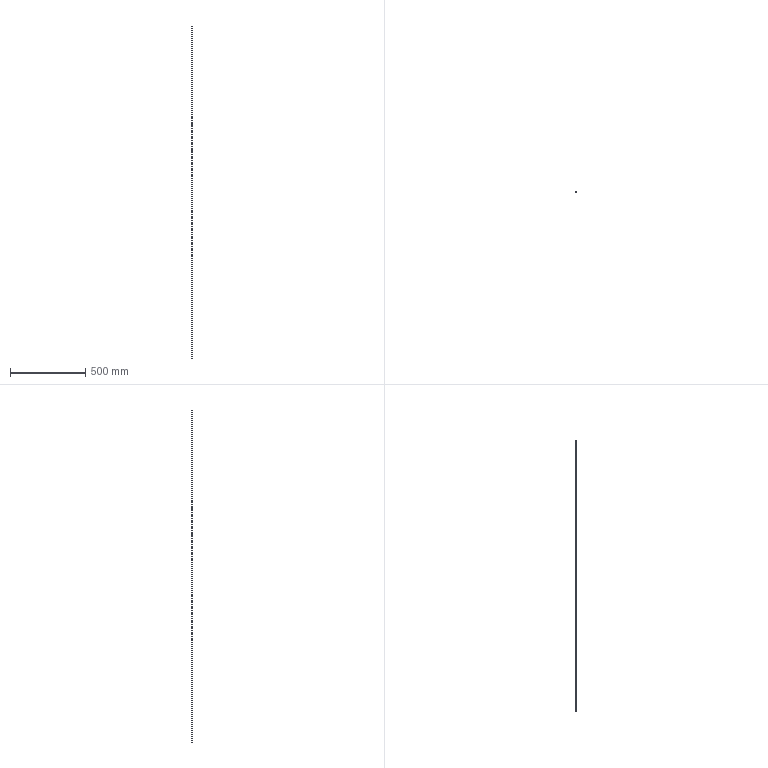Part | STEP file | P2 | 1 solid | 3 faces | box 4 x 4 x 2200 mm | volume 27646 mm3 | plane 2 | cylinder 1 | commonest cylinder face diameters 4 x1
STEP:
#1=CARTESIAN_POINT('',(0.,0.,0.));
#2=DIRECTION('',(0.,0.,1.));
#3=DIRECTION('',(1.,0.,0.));
#4=AXIS2_PLACEMENT_3D('',#1,#2,#3);
#5=CARTESIAN_POINT('',(2.,0.,2200.));
#6=VERTEX_POINT('',#5);
#7=CARTESIAN_POINT('',(0.,0.,2200.));
#8=DIRECTION('',(0.,0.,-1.));
#9=DIRECTION('',(-1.,0.,0.));
#10=AXIS2_PLACEMENT_3D('',#7,#8,#9);
#11=CIRCLE('',#10,2.);
#12=CARTESIAN_POINT('',(0.,0.,0.));
#13=DIRECTION('',(0.,0.,1.));
#14=DIRECTION('',(-1.,0.,0.));
#15=AXIS2_PLACEMENT_3D('',#12,#13,#14);
#16=CYLINDRICAL_SURFACE('',#15,2.);
#17=CARTESIAN_POINT('',(12.566,2200.));
#18=DIRECTION('',(-1.,0.));
#19=VECTOR('',#18,1.);
#20=LINE('',#17,#19);
#21=(GEOMETRIC_REPRESENTATION_CONTEXT(2)PARAMETRIC_REPRESENTATION_CONTEXT()REPRESENTATION_CONTEXT('',''));
#22=DEFINITIONAL_REPRESENTATION('',(#20),#21);
#23=PCURVE('',#16,#22);
#24=CARTESIAN_POINT('',(0.,0.,2200.));
#25=DIRECTION('',(0.,0.,1.));
#26=DIRECTION('',(1.,0.,0.));
#27=AXIS2_PLACEMENT_3D('',#24,#25,#26);
#28=PLANE('',#27);
#29=CARTESIAN_POINT('',(-2.,0.));
#30=CARTESIAN_POINT('',(-2.,3.464));
#31=CARTESIAN_POINT('',(1.,1.732));
#32=CARTESIAN_POINT('',(4.,0.));
#33=CARTESIAN_POINT('',(1.,-1.732));
#34=CARTESIAN_POINT('',(-2.,-3.464));
#35=CARTESIAN_POINT('',(-2.,0.));
#36=(BOUNDED_CURVE()B_SPLINE_CURVE(2,(#29,#30,#31,#32,#33,#34,#35),.UNSPECIFIED.,.T.,.F.)B_SPLINE_CURVE_WITH_KNOTS((1,2,2,2,2,1),(-2.094,0.,2.094,4.189,6.283,8.378),.UNSPECIFIED.)CURVE()GEOMETRIC_REPRESENTATION_ITEM()RATIONAL_B_SPLINE_CURVE((1.,0.5,1.,0.5,1.,0.5,1.))REPRESENTATION_ITEM(''));
#37=(GEOMETRIC_REPRESENTATION_CONTEXT(2)PARAMETRIC_REPRESENTATION_CONTEXT()REPRESENTATION_CONTEXT('',''));
#38=DEFINITIONAL_REPRESENTATION('',(#36),#37);
#39=PCURVE('',#28,#38);
#40=SURFACE_CURVE('',#11,(#23,#39),.PCURVE_S1.);
#41=EDGE_CURVE('',#6,#6,#40,.T.);
#42=ORIENTED_EDGE('',*,*,#41,.T.);
#43=CARTESIAN_POINT('',(2.,0.,0.));
#44=VERTEX_POINT('',#43);
#45=CARTESIAN_POINT('',(2.,0.,0.));
#46=CARTESIAN_POINT('',(2.,0.,2200.));
#47=B_SPLINE_CURVE_WITH_KNOTS('',1,(#45,#46),.UNSPECIFIED.,.F.,.F.,(2,2),(0.,2200.),.PIECEWISE_BEZIER_KNOTS.);
#48=CARTESIAN_POINT('',(3.142,0.));
#49=DIRECTION('',(0.,1.));
#50=VECTOR('',#49,1.);
#51=LINE('',#48,#50);
#52=(GEOMETRIC_REPRESENTATION_CONTEXT(2)PARAMETRIC_REPRESENTATION_CONTEXT()REPRESENTATION_CONTEXT('',''));
#53=DEFINITIONAL_REPRESENTATION('',(#51),#52);
#54=PCURVE('',#16,#53);
#55=CARTESIAN_POINT('',(9.425,0.));
#56=DIRECTION('',(0.,1.));
#57=VECTOR('',#56,1.);
#58=LINE('',#55,#57);
#59=(GEOMETRIC_REPRESENTATION_CONTEXT(2)PARAMETRIC_REPRESENTATION_CONTEXT()REPRESENTATION_CONTEXT('',''));
#60=DEFINITIONAL_REPRESENTATION('',(#58),#59);
#61=PCURVE('',#16,#60);
#62=SEAM_CURVE('',#47,(#54,#61),.PCURVE_S1.);
#63=EDGE_CURVE('',#44,#6,#62,.T.);
#64=ORIENTED_EDGE('',*,*,#63,.F.);
#65=CARTESIAN_POINT('',(0.,0.,0.));
#66=DIRECTION('',(0.,0.,-1.));
#67=DIRECTION('',(-1.,0.,0.));
#68=AXIS2_PLACEMENT_3D('',#65,#66,#67);
#69=CIRCLE('',#68,2.);
#70=CARTESIAN_POINT('',(12.566,0.));
#71=DIRECTION('',(-1.,0.));
#72=VECTOR('',#71,1.);
#73=LINE('',#70,#72);
#74=(GEOMETRIC_REPRESENTATION_CONTEXT(2)PARAMETRIC_REPRESENTATION_CONTEXT()REPRESENTATION_CONTEXT('',''));
#75=DEFINITIONAL_REPRESENTATION('',(#73),#74);
#76=PCURVE('',#16,#75);
#77=CARTESIAN_POINT('',(0.,0.,0.));
#78=DIRECTION('',(0.,0.,1.));
#79=DIRECTION('',(1.,0.,0.));
#80=AXIS2_PLACEMENT_3D('',#77,#78,#79);
#81=PLANE('',#80);
#82=CARTESIAN_POINT('',(-2.,0.));
#83=CARTESIAN_POINT('',(-2.,3.464));
#84=CARTESIAN_POINT('',(1.,1.732));
#85=CARTESIAN_POINT('',(4.,0.));
#86=CARTESIAN_POINT('',(1.,-1.732));
#87=CARTESIAN_POINT('',(-2.,-3.464));
#88=CARTESIAN_POINT('',(-2.,0.));
#89=(BOUNDED_CURVE()B_SPLINE_CURVE(2,(#82,#83,#84,#85,#86,#87,#88),.UNSPECIFIED.,.T.,.F.)B_SPLINE_CURVE_WITH_KNOTS((1,2,2,2,2,1),(-2.094,0.,2.094,4.189,6.283,8.378),.UNSPECIFIED.)CURVE()GEOMETRIC_REPRESENTATION_ITEM()RATIONAL_B_SPLINE_CURVE((1.,0.5,1.,0.5,1.,0.5,1.))REPRESENTATION_ITEM(''));
#90=(GEOMETRIC_REPRESENTATION_CONTEXT(2)PARAMETRIC_REPRESENTATION_CONTEXT()REPRESENTATION_CONTEXT('',''));
#91=DEFINITIONAL_REPRESENTATION('',(#89),#90);
#92=PCURVE('',#81,#91);
#93=SURFACE_CURVE('',#69,(#76,#92),.PCURVE_S1.);
#94=EDGE_CURVE('',#44,#44,#93,.T.);
#95=ORIENTED_EDGE('',*,*,#94,.F.);
#96=ORIENTED_EDGE('',*,*,#63,.T.);
#97=EDGE_LOOP('',(#42,#64,#95,#96));
#98=FACE_BOUND('',#97,.T.);
#99=ADVANCED_FACE('',(#98),#16,.T.);
#100=ORIENTED_EDGE('',*,*,#94,.T.);
#101=EDGE_LOOP('',(#100));
#102=FACE_BOUND('',#101,.T.);
#103=ADVANCED_FACE('',(#102),#81,.F.);
#104=ORIENTED_EDGE('',*,*,#41,.F.);
#105=EDGE_LOOP('',(#104));
#106=FACE_BOUND('',#105,.T.);
#107=ADVANCED_FACE('',(#106),#28,.T.);
#108=CLOSED_SHELL('',(#99,#103,#107));
#109=MANIFOLD_SOLID_BREP('',#108);
#110=(LENGTH_UNIT()NAMED_UNIT(*)SI_UNIT(.MILLI.,.METRE.));
#111=UNCERTAINTY_MEASURE_WITH_UNIT(LENGTH_MEASURE(0.00001),#110,'','');
#112=(NAMED_UNIT(*)PLANE_ANGLE_UNIT()SI_UNIT($,.RADIAN.));
#113=(NAMED_UNIT(*)SI_UNIT($,.STERADIAN.)SOLID_ANGLE_UNIT());
#114=(GEOMETRIC_REPRESENTATION_CONTEXT(3)GLOBAL_UNCERTAINTY_ASSIGNED_CONTEXT((#111))GLOBAL_UNIT_ASSIGNED_CONTEXT((#110,#112,#113))REPRESENTATION_CONTEXT('',''));
#115=ADVANCED_BREP_SHAPE_REPRESENTATION('',(#4,#109),#114);